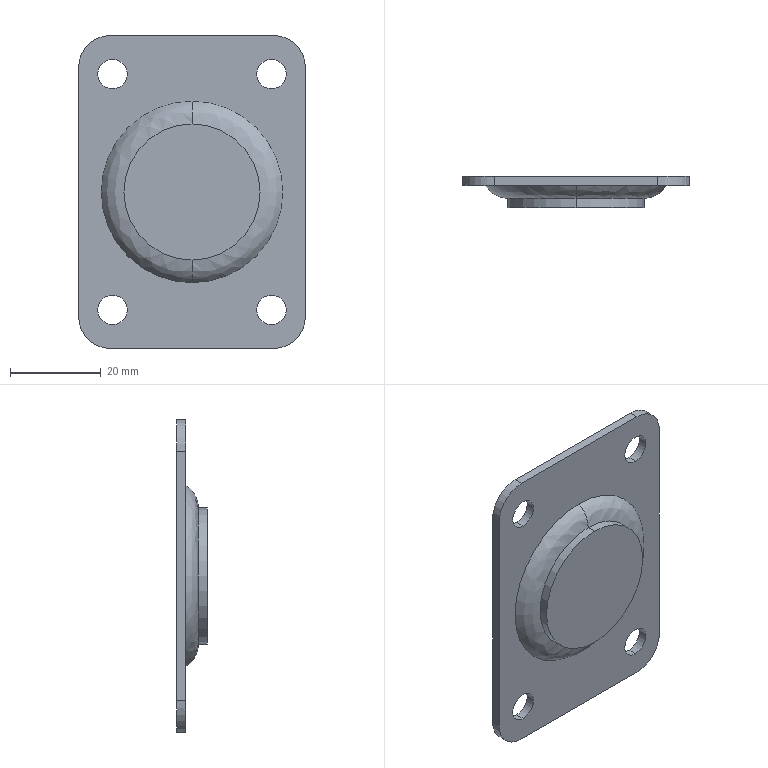Part | STEP file | Caster plate | 1 solid | 46 faces | box 50 x 6.8 x 69 mm | volume 8896 mm3 | cylinder 20 | torus 10 | plane 10 | spline 6 | commonest cylinder face diameters 6.5 x8 14 x4 16 x2 20 x2 30 x2 36 x2
STEP:
#1=CARTESIAN_POINT('',(0.,4.8,20.));
#2=VERTEX_POINT('',#1);
#3=CARTESIAN_POINT('',(0.,4.8,-20.));
#4=VERTEX_POINT('',#3);
#5=CARTESIAN_POINT('',(0.,4.8,0.));
#6=DIRECTION('',(0.,-1.,0.));
#7=DIRECTION('',(0.,0.,1.));
#8=AXIS2_PLACEMENT_3D('',#5,#6,#7);
#9=CIRCLE('',#8,20.);
#10=EDGE_CURVE('',#2,#4,#9,.T.);
#11=ORIENTED_EDGE('',*,*,#10,.T.);
#12=CARTESIAN_POINT('',(0.,2.,-15.));
#13=VERTEX_POINT('',#12);
#14=CARTESIAN_POINT('',(0.,7.864,-15.));
#15=DIRECTION('',(-1.,0.,0.));
#16=DIRECTION('',(0.,0.,-1.));
#17=AXIS2_PLACEMENT_3D('',#14,#15,#16);
#18=CIRCLE('',#17,5.864);
#19=EDGE_CURVE('',#4,#13,#18,.T.);
#20=ORIENTED_EDGE('',*,*,#19,.T.);
#21=CARTESIAN_POINT('',(0.,2.,15.));
#22=VERTEX_POINT('',#21);
#23=CARTESIAN_POINT('',(0.,2.,0.));
#24=DIRECTION('',(0.,1.,0.));
#25=DIRECTION('',(0.,0.,1.));
#26=AXIS2_PLACEMENT_3D('',#23,#24,#25);
#27=CIRCLE('',#26,15.);
#28=EDGE_CURVE('',#13,#22,#27,.T.);
#29=ORIENTED_EDGE('',*,*,#28,.T.);
#30=CARTESIAN_POINT('',(0.,7.864,15.));
#31=DIRECTION('',(1.,0.,0.));
#32=DIRECTION('',(0.,0.,1.));
#33=AXIS2_PLACEMENT_3D('',#30,#31,#32);
#34=CIRCLE('',#33,5.864);
#35=EDGE_CURVE('',#2,#22,#34,.T.);
#36=ORIENTED_EDGE('',*,*,#35,.F.);
#37=EDGE_LOOP('',(#11,#20,#29,#36));
#38=FACE_OUTER_BOUND('',#37,.T.);
#39=CARTESIAN_POINT('',(0.,4.8,-20.));
#40=CARTESIAN_POINT('',(-40.,4.8,-20.));
#41=CARTESIAN_POINT('',(-40.,4.8,20.));
#42=CARTESIAN_POINT('',(0.,4.8,20.));
#43=CARTESIAN_POINT('',(0.,3.02,-18.909));
#44=CARTESIAN_POINT('',(-37.818,3.02,-18.909));
#45=CARTESIAN_POINT('',(-37.818,3.02,18.909));
#46=CARTESIAN_POINT('',(0.,3.02,18.909));
#47=CARTESIAN_POINT('',(0.,2.,-17.088));
#48=CARTESIAN_POINT('',(-34.175,2.,-17.088));
#49=CARTESIAN_POINT('',(-34.175,2.,17.088));
#50=CARTESIAN_POINT('',(0.,2.,17.088));
#51=CARTESIAN_POINT('',(0.,2.,-15.));
#52=CARTESIAN_POINT('',(-30.,2.,-15.));
#53=CARTESIAN_POINT('',(-30.,2.,15.));
#54=CARTESIAN_POINT('',(0.,2.,15.));
#55=(BOUNDED_SURFACE()B_SPLINE_SURFACE(3,3,((#39,#40,#41,#42),(#43,#44,#45,#46),(#47,#48,#49,#50),(#51,#52,#53,#54)),.UNSPECIFIED.,.F.,.F.,.F.)B_SPLINE_SURFACE_WITH_KNOTS((4,4),(4,4),(0.,1.),(0.,1.),.UNSPECIFIED.)GEOMETRIC_REPRESENTATION_ITEM()RATIONAL_B_SPLINE_SURFACE(((1.,0.3333,0.3333,1.),(0.915,0.305,0.305,0.915),(0.915,0.305,0.305,0.915),(1.,0.3333,0.3333,1.)))REPRESENTATION_ITEM('')SURFACE());
#56=ADVANCED_FACE('',(#38),#55,.T.);
#57=CARTESIAN_POINT('',(0.,3.8,15.5));
#58=VERTEX_POINT('',#57);
#59=CARTESIAN_POINT('',(0.,3.8,-15.5));
#60=VERTEX_POINT('',#59);
#61=CARTESIAN_POINT('',(0.,3.8,15.5));
#62=CARTESIAN_POINT('',(31.,3.8,15.5));
#63=CARTESIAN_POINT('',(31.,3.8,-15.5));
#64=CARTESIAN_POINT('',(0.,3.8,-15.5));
#65=(BOUNDED_CURVE()B_SPLINE_CURVE(3,(#61,#62,#63,#64),.UNSPECIFIED.,.F.,.T.)B_SPLINE_CURVE_WITH_KNOTS((4,4),(0.,0.5),.UNSPECIFIED.)CURVE()GEOMETRIC_REPRESENTATION_ITEM()RATIONAL_B_SPLINE_CURVE((1.,0.3333,0.3333,1.))REPRESENTATION_ITEM(''));
#66=EDGE_CURVE('',#58,#60,#65,.T.);
#67=ORIENTED_EDGE('',*,*,#66,.T.);
#68=CARTESIAN_POINT('',(0.,4.3,-15.));
#69=VERTEX_POINT('',#68);
#70=CARTESIAN_POINT('',(0.,4.3,-15.5));
#71=DIRECTION('',(-1.,0.,0.));
#72=DIRECTION('',(0.,0.,-1.));
#73=AXIS2_PLACEMENT_3D('',#70,#71,#72);
#74=CIRCLE('',#73,0.5);
#75=EDGE_CURVE('',#60,#69,#74,.T.);
#76=ORIENTED_EDGE('',*,*,#75,.T.);
#77=CARTESIAN_POINT('',(0.,4.3,15.));
#78=VERTEX_POINT('',#77);
#79=CARTESIAN_POINT('',(0.,4.3,0.));
#80=DIRECTION('',(0.,1.,0.));
#81=DIRECTION('',(0.,0.,1.));
#82=AXIS2_PLACEMENT_3D('',#79,#80,#81);
#83=CIRCLE('',#82,15.);
#84=EDGE_CURVE('',#78,#69,#83,.T.);
#85=ORIENTED_EDGE('',*,*,#84,.F.);
#86=CARTESIAN_POINT('',(0.,4.3,15.5));
#87=DIRECTION('',(1.,0.,0.));
#88=DIRECTION('',(0.,0.,1.));
#89=AXIS2_PLACEMENT_3D('',#86,#87,#88);
#90=CIRCLE('',#89,0.5);
#91=EDGE_CURVE('',#58,#78,#90,.T.);
#92=ORIENTED_EDGE('',*,*,#91,.F.);
#93=EDGE_LOOP('',(#67,#76,#85,#92));
#94=FACE_OUTER_BOUND('',#93,.T.);
#95=CARTESIAN_POINT('',(0.,3.8,15.5));
#96=CARTESIAN_POINT('',(31.,3.8,15.5));
#97=CARTESIAN_POINT('',(31.,3.8,-15.5));
#98=CARTESIAN_POINT('',(0.,3.8,-15.5));
#99=CARTESIAN_POINT('',(0.,3.8,15.207));
#100=CARTESIAN_POINT('',(30.414,3.8,15.207));
#101=CARTESIAN_POINT('',(30.414,3.8,-15.207));
#102=CARTESIAN_POINT('',(0.,3.8,-15.207));
#103=CARTESIAN_POINT('',(0.,4.007,15.));
#104=CARTESIAN_POINT('',(30.,4.007,15.));
#105=CARTESIAN_POINT('',(30.,4.007,-15.));
#106=CARTESIAN_POINT('',(0.,4.007,-15.));
#107=CARTESIAN_POINT('',(0.,4.3,15.));
#108=CARTESIAN_POINT('',(30.,4.3,15.));
#109=CARTESIAN_POINT('',(30.,4.3,-15.));
#110=CARTESIAN_POINT('',(0.,4.3,-15.));
#111=(BOUNDED_SURFACE()B_SPLINE_SURFACE(3,3,((#95,#96,#97,#98),(#99,#100,#101,#102),(#103,#104,#105,#106),(#107,#108,#109,#110)),.UNSPECIFIED.,.F.,.F.,.T.)B_SPLINE_SURFACE_WITH_KNOTS((4,4),(4,4),(0.,1.),(0.,1.),.UNSPECIFIED.)GEOMETRIC_REPRESENTATION_ITEM()RATIONAL_B_SPLINE_SURFACE(((1.,0.3333,0.3333,1.),(0.8047,0.2682,0.2682,0.8047),(0.8047,0.2682,0.2682,0.8047),(1.,0.3333,0.3333,1.)))REPRESENTATION_ITEM('')SURFACE());
#112=ADVANCED_FACE('',(#94),#111,.F.);
#113=CARTESIAN_POINT('',(0.,4.3,10.));
#114=VERTEX_POINT('',#113);
#115=CARTESIAN_POINT('',(0.,4.3,-10.));
#116=VERTEX_POINT('',#115);
#117=CARTESIAN_POINT('',(0.,4.3,0.));
#118=DIRECTION('',(0.,-1.,0.));
#119=DIRECTION('',(0.,0.,1.));
#120=AXIS2_PLACEMENT_3D('',#117,#118,#119);
#121=CIRCLE('',#120,10.);
#122=EDGE_CURVE('',#114,#116,#121,.T.);
#123=ORIENTED_EDGE('',*,*,#122,.T.);
#124=CARTESIAN_POINT('',(0.,2.546,-12.5));
#125=DIRECTION('',(-1.,0.,0.));
#126=DIRECTION('',(0.,0.,-1.));
#127=AXIS2_PLACEMENT_3D('',#124,#125,#126);
#128=CIRCLE('',#127,3.054);
#129=EDGE_CURVE('',#116,#69,#128,.T.);
#130=ORIENTED_EDGE('',*,*,#129,.T.);
#131=CARTESIAN_POINT('',(0.,4.3,0.));
#132=DIRECTION('',(0.,1.,0.));
#133=DIRECTION('',(0.,0.,1.));
#134=AXIS2_PLACEMENT_3D('',#131,#132,#133);
#135=CIRCLE('',#134,15.);
#136=EDGE_CURVE('',#69,#78,#135,.T.);
#137=ORIENTED_EDGE('',*,*,#136,.T.);
#138=CARTESIAN_POINT('',(0.,2.546,12.5));
#139=DIRECTION('',(1.,0.,0.));
#140=DIRECTION('',(0.,0.,1.));
#141=AXIS2_PLACEMENT_3D('',#138,#139,#140);
#142=CIRCLE('',#141,3.054);
#143=EDGE_CURVE('',#114,#78,#142,.T.);
#144=ORIENTED_EDGE('',*,*,#143,.F.);
#145=EDGE_LOOP('',(#123,#130,#137,#144));
#146=FACE_OUTER_BOUND('',#145,.T.);
#147=CARTESIAN_POINT('',(0.,4.3,-10.));
#148=CARTESIAN_POINT('',(-20.,4.3,-10.));
#149=CARTESIAN_POINT('',(-20.,4.3,10.));
#150=CARTESIAN_POINT('',(0.,4.3,10.));
#151=CARTESIAN_POINT('',(0.,6.205,-11.336));
#152=CARTESIAN_POINT('',(-22.673,6.205,-11.336));
#153=CARTESIAN_POINT('',(-22.673,6.205,11.336));
#154=CARTESIAN_POINT('',(0.,6.205,11.336));
#155=CARTESIAN_POINT('',(0.,6.205,-13.664));
#156=CARTESIAN_POINT('',(-27.327,6.205,-13.664));
#157=CARTESIAN_POINT('',(-27.327,6.205,13.664));
#158=CARTESIAN_POINT('',(0.,6.205,13.664));
#159=CARTESIAN_POINT('',(0.,4.3,-15.));
#160=CARTESIAN_POINT('',(-30.,4.3,-15.));
#161=CARTESIAN_POINT('',(-30.,4.3,15.));
#162=CARTESIAN_POINT('',(0.,4.3,15.));
#163=(BOUNDED_SURFACE()B_SPLINE_SURFACE(3,3,((#147,#148,#149,#150),(#151,#152,#153,#154),(#155,#156,#157,#158),(#159,#160,#161,#162)),.UNSPECIFIED.,.F.,.F.,.F.)B_SPLINE_SURFACE_WITH_KNOTS((4,4),(4,4),(0.,1.),(0.,1.),.UNSPECIFIED.)GEOMETRIC_REPRESENTATION_ITEM()RATIONAL_B_SPLINE_SURFACE(((1.,0.3333,0.3333,1.),(0.7162,0.2387,0.2387,0.7162),(0.7162,0.2387,0.2387,0.7162),(1.,0.3333,0.3333,1.)))REPRESENTATION_ITEM('')SURFACE());
#164=ADVANCED_FACE('',(#146),#163,.T.);
#165=CARTESIAN_POINT('',(0.,6.8,-20.));
#166=VERTEX_POINT('',#165);
#167=CARTESIAN_POINT('',(0.,6.8,20.));
#168=VERTEX_POINT('',#167);
#169=CARTESIAN_POINT('',(0.,6.8,0.));
#170=DIRECTION('',(0.,-1.,0.));
#171=DIRECTION('',(0.,0.,1.));
#172=AXIS2_PLACEMENT_3D('',#169,#170,#171);
#173=CIRCLE('',#172,20.);
#174=EDGE_CURVE('',#166,#168,#173,.T.);
#175=ORIENTED_EDGE('',*,*,#174,.F.);
#176=CARTESIAN_POINT('',(0.,4.8,-18.));
#177=VERTEX_POINT('',#176);
#178=CARTESIAN_POINT('',(0.,4.8,-20.));
#179=DIRECTION('',(1.,0.,0.));
#180=DIRECTION('',(0.,0.,-1.));
#181=AXIS2_PLACEMENT_3D('',#178,#179,#180);
#182=CIRCLE('',#181,2.);
#183=EDGE_CURVE('',#166,#177,#182,.T.);
#184=ORIENTED_EDGE('',*,*,#183,.T.);
#185=CARTESIAN_POINT('',(0.,4.8,18.));
#186=VERTEX_POINT('',#185);
#187=CARTESIAN_POINT('',(0.,4.8,0.));
#188=DIRECTION('',(0.,1.,0.));
#189=DIRECTION('',(0.,0.,1.));
#190=AXIS2_PLACEMENT_3D('',#187,#188,#189);
#191=CIRCLE('',#190,18.);
#192=EDGE_CURVE('',#186,#177,#191,.T.);
#193=ORIENTED_EDGE('',*,*,#192,.F.);
#194=CARTESIAN_POINT('',(0.,4.8,20.));
#195=DIRECTION('',(-1.,0.,0.));
#196=DIRECTION('',(0.,0.,1.));
#197=AXIS2_PLACEMENT_3D('',#194,#195,#196);
#198=CIRCLE('',#197,2.);
#199=EDGE_CURVE('',#168,#186,#198,.T.);
#200=ORIENTED_EDGE('',*,*,#199,.F.);
#201=EDGE_LOOP('',(#175,#184,#193,#200));
#202=FACE_OUTER_BOUND('',#201,.T.);
#203=CARTESIAN_POINT('',(0.,4.8,0.));
#204=DIRECTION('',(0.,1.,0.));
#205=DIRECTION('',(0.,0.,1.));
#206=AXIS2_PLACEMENT_3D('',#203,#204,#205);
#207=TOROIDAL_SURFACE('',#206,20.,2.);
#208=ADVANCED_FACE('',(#202),#207,.T.);
#209=CARTESIAN_POINT('',(0.,5.8,-8.));
#210=VERTEX_POINT('',#209);
#211=CARTESIAN_POINT('',(0.,5.8,8.));
#212=VERTEX_POINT('',#211);
#213=CARTESIAN_POINT('',(0.,5.8,0.));
#214=DIRECTION('',(0.,-1.,0.));
#215=DIRECTION('',(0.,0.,1.));
#216=AXIS2_PLACEMENT_3D('',#213,#214,#215);
#217=CIRCLE('',#216,8.);
#218=EDGE_CURVE('',#210,#212,#217,.T.);
#219=ORIENTED_EDGE('',*,*,#218,.F.);
#220=CARTESIAN_POINT('',(0.,6.8,-7.));
#221=VERTEX_POINT('',#220);
#222=CARTESIAN_POINT('',(0.,5.8,-7.));
#223=DIRECTION('',(1.,0.,0.));
#224=DIRECTION('',(0.,0.,-1.));
#225=AXIS2_PLACEMENT_3D('',#222,#223,#224);
#226=CIRCLE('',#225,1.);
#227=EDGE_CURVE('',#210,#221,#226,.T.);
#228=ORIENTED_EDGE('',*,*,#227,.T.);
#229=CARTESIAN_POINT('',(0.,6.8,7.));
#230=VERTEX_POINT('',#229);
#231=CARTESIAN_POINT('',(0.,6.8,0.));
#232=DIRECTION('',(0.,1.,0.));
#233=DIRECTION('',(0.,0.,1.));
#234=AXIS2_PLACEMENT_3D('',#231,#232,#233);
#235=CIRCLE('',#234,7.);
#236=EDGE_CURVE('',#230,#221,#235,.T.);
#237=ORIENTED_EDGE('',*,*,#236,.F.);
#238=CARTESIAN_POINT('',(0.,5.8,7.));
#239=DIRECTION('',(-1.,0.,0.));
#240=DIRECTION('',(0.,0.,1.));
#241=AXIS2_PLACEMENT_3D('',#238,#239,#240);
#242=CIRCLE('',#241,1.);
#243=EDGE_CURVE('',#212,#230,#242,.T.);
#244=ORIENTED_EDGE('',*,*,#243,.F.);
#245=EDGE_LOOP('',(#219,#228,#237,#244));
#246=FACE_OUTER_BOUND('',#245,.T.);
#247=CARTESIAN_POINT('',(0.,5.8,0.));
#248=DIRECTION('',(0.,1.,0.));
#249=DIRECTION('',(0.,0.,1.));
#250=AXIS2_PLACEMENT_3D('',#247,#248,#249);
#251=TOROIDAL_SURFACE('',#250,7.,1.);
#252=ADVANCED_FACE('',(#246),#251,.T.);
#253=CARTESIAN_POINT('',(0.,4.3,18.));
#254=VERTEX_POINT('',#253);
#255=CARTESIAN_POINT('',(0.,4.3,-18.));
#256=VERTEX_POINT('',#255);
#257=CARTESIAN_POINT('',(0.,4.3,0.));
#258=DIRECTION('',(0.,-1.,0.));
#259=DIRECTION('',(0.,0.,-1.));
#260=AXIS2_PLACEMENT_3D('',#257,#258,#259);
#261=CIRCLE('',#260,18.);
#262=EDGE_CURVE('',#254,#256,#261,.T.);
#263=ORIENTED_EDGE('',*,*,#262,.F.);
#264=CARTESIAN_POINT('',(0.,3.8,17.5));
#265=VERTEX_POINT('',#264);
#266=CARTESIAN_POINT('',(0.,4.3,17.5));
#267=DIRECTION('',(1.,0.,0.));
#268=DIRECTION('',(0.,0.,-1.));
#269=AXIS2_PLACEMENT_3D('',#266,#267,#268);
#270=CIRCLE('',#269,0.5);
#271=EDGE_CURVE('',#254,#265,#270,.T.);
#272=ORIENTED_EDGE('',*,*,#271,.T.);
#273=CARTESIAN_POINT('',(0.,3.8,-17.5));
#274=VERTEX_POINT('',#273);
#275=CARTESIAN_POINT('',(0.,3.8,0.));
#276=DIRECTION('',(0.,1.,0.));
#277=DIRECTION('',(0.,0.,-1.));
#278=AXIS2_PLACEMENT_3D('',#275,#276,#277);
#279=CIRCLE('',#278,17.5);
#280=EDGE_CURVE('',#274,#265,#279,.T.);
#281=ORIENTED_EDGE('',*,*,#280,.F.);
#282=CARTESIAN_POINT('',(0.,4.3,-17.5));
#283=DIRECTION('',(-1.,0.,0.));
#284=DIRECTION('',(0.,0.,1.));
#285=AXIS2_PLACEMENT_3D('',#282,#283,#284);
#286=CIRCLE('',#285,0.5);
#287=EDGE_CURVE('',#256,#274,#286,.T.);
#288=ORIENTED_EDGE('',*,*,#287,.F.);
#289=EDGE_LOOP('',(#263,#272,#281,#288));
#290=FACE_OUTER_BOUND('',#289,.T.);
#291=CARTESIAN_POINT('',(0.,4.3,0.));
#292=DIRECTION('',(0.,-1.,0.));
#293=DIRECTION('',(0.,0.,-1.));
#294=AXIS2_PLACEMENT_3D('',#291,#292,#293);
#295=TOROIDAL_SURFACE('',#294,17.5,0.5);
#296=ADVANCED_FACE('',(#290),#295,.F.);
#297=CARTESIAN_POINT('',(0.,2.8,8.5));
#298=VERTEX_POINT('',#297);
#299=CARTESIAN_POINT('',(0.,2.8,-8.5));
#300=VERTEX_POINT('',#299);
#301=CARTESIAN_POINT('',(0.,2.8,0.));
#302=DIRECTION('',(0.,-1.,0.));
#303=DIRECTION('',(0.,0.,-1.));
#304=AXIS2_PLACEMENT_3D('',#301,#302,#303);
#305=CIRCLE('',#304,8.5);
#306=EDGE_CURVE('',#298,#300,#305,.T.);
#307=ORIENTED_EDGE('',*,*,#306,.F.);
#308=CARTESIAN_POINT('',(0.,3.3,8.));
#309=VERTEX_POINT('',#308);
#310=CARTESIAN_POINT('',(0.,3.3,8.5));
#311=DIRECTION('',(1.,0.,0.));
#312=DIRECTION('',(0.,0.,-1.));
#313=AXIS2_PLACEMENT_3D('',#310,#311,#312);
#314=CIRCLE('',#313,0.5);
#315=EDGE_CURVE('',#298,#309,#314,.T.);
#316=ORIENTED_EDGE('',*,*,#315,.T.);
#317=CARTESIAN_POINT('',(0.,3.3,-8.));
#318=VERTEX_POINT('',#317);
#319=CARTESIAN_POINT('',(0.,3.3,0.));
#320=DIRECTION('',(0.,1.,0.));
#321=DIRECTION('',(0.,0.,-1.));
#322=AXIS2_PLACEMENT_3D('',#319,#320,#321);
#323=CIRCLE('',#322,8.);
#324=EDGE_CURVE('',#318,#309,#323,.T.);
#325=ORIENTED_EDGE('',*,*,#324,.F.);
#326=CARTESIAN_POINT('',(0.,3.3,-8.5));
#327=DIRECTION('',(-1.,0.,0.));
#328=DIRECTION('',(0.,0.,1.));
#329=AXIS2_PLACEMENT_3D('',#326,#327,#328);
#330=CIRCLE('',#329,0.5);
#331=EDGE_CURVE('',#300,#318,#330,.T.);
#332=ORIENTED_EDGE('',*,*,#331,.F.);
#333=EDGE_LOOP('',(#307,#316,#325,#332));
#334=FACE_OUTER_BOUND('',#333,.T.);
#335=CARTESIAN_POINT('',(0.,3.3,0.));
#336=DIRECTION('',(0.,-1.,0.));
#337=DIRECTION('',(0.,0.,-1.));
#338=AXIS2_PLACEMENT_3D('',#335,#336,#337);
#339=TOROIDAL_SURFACE('',#338,8.5,0.5);
#340=ADVANCED_FACE('',(#334),#339,.F.);
#341=CARTESIAN_POINT('',(0.,3.3,10.));
#342=VERTEX_POINT('',#341);
#343=CARTESIAN_POINT('',(0.,3.3,-10.));
#344=VERTEX_POINT('',#343);
#345=CARTESIAN_POINT('',(0.,3.3,0.));
#346=DIRECTION('',(0.,-1.,0.));
#347=DIRECTION('',(0.,0.,-1.));
#348=AXIS2_PLACEMENT_3D('',#345,#346,#347);
#349=CIRCLE('',#348,10.);
#350=EDGE_CURVE('',#342,#344,#349,.T.);
#351=ORIENTED_EDGE('',*,*,#350,.F.);
#352=CARTESIAN_POINT('',(0.,2.8,9.5));
#353=VERTEX_POINT('',#352);
#354=CARTESIAN_POINT('',(0.,3.3,9.5));
#355=DIRECTION('',(1.,0.,0.));
#356=DIRECTION('',(0.,0.,-1.));
#357=AXIS2_PLACEMENT_3D('',#354,#355,#356);
#358=CIRCLE('',#357,0.5);
#359=EDGE_CURVE('',#342,#353,#358,.T.);
#360=ORIENTED_EDGE('',*,*,#359,.T.);
#361=CARTESIAN_POINT('',(0.,2.8,-9.5));
#362=VERTEX_POINT('',#361);
#363=CARTESIAN_POINT('',(0.,2.8,0.));
#364=DIRECTION('',(0.,1.,0.));
#365=DIRECTION('',(0.,0.,-1.));
#366=AXIS2_PLACEMENT_3D('',#363,#364,#365);
#367=CIRCLE('',#366,9.5);
#368=EDGE_CURVE('',#362,#353,#367,.T.);
#369=ORIENTED_EDGE('',*,*,#368,.F.);
#370=CARTESIAN_POINT('',(0.,3.3,-9.5));
#371=DIRECTION('',(-1.,0.,0.));
#372=DIRECTION('',(0.,0.,1.));
#373=AXIS2_PLACEMENT_3D('',#370,#371,#372);
#374=CIRCLE('',#373,0.5);
#375=EDGE_CURVE('',#344,#362,#374,.T.);
#376=ORIENTED_EDGE('',*,*,#375,.F.);
#377=EDGE_LOOP('',(#351,#360,#369,#376));
#378=FACE_OUTER_BOUND('',#377,.T.);
#379=CARTESIAN_POINT('',(0.,3.3,0.));
#380=DIRECTION('',(0.,-1.,0.));
#381=DIRECTION('',(0.,0.,-1.));
#382=AXIS2_PLACEMENT_3D('',#379,#380,#381);
#383=TOROIDAL_SURFACE('',#382,9.5,0.5);
#384=ADVANCED_FACE('',(#378),#383,.F.);
#385=CARTESIAN_POINT('',(17.5,6.8,-22.75));
#386=VERTEX_POINT('',#385);
#387=CARTESIAN_POINT('',(17.5,6.8,-29.25));
#388=VERTEX_POINT('',#387);
#389=CARTESIAN_POINT('',(17.5,6.8,-26.));
#390=DIRECTION('',(0.,-1.,0.));
#391=DIRECTION('',(0.,0.,-1.));
#392=AXIS2_PLACEMENT_3D('',#389,#390,#391);
#393=CIRCLE('',#392,3.25);
#394=EDGE_CURVE('',#386,#388,#393,.T.);
#395=ORIENTED_EDGE('',*,*,#394,.F.);
#396=CARTESIAN_POINT('',(17.5,4.8,-22.75));
#397=VERTEX_POINT('',#396);
#398=CARTESIAN_POINT('',(17.5,4.8,-22.75));
#399=DIRECTION('',(0.,-1.,0.));
#400=VECTOR('',#399,1000.);
#401=LINE('',#398,#400);
#402=EDGE_CURVE('',#386,#397,#401,.T.);
#403=ORIENTED_EDGE('',*,*,#402,.T.);
#404=CARTESIAN_POINT('',(17.5,4.8,-29.25));
#405=VERTEX_POINT('',#404);
#406=CARTESIAN_POINT('',(17.5,4.8,-26.));
#407=DIRECTION('',(0.,-1.,0.));
#408=DIRECTION('',(0.,0.,-1.));
#409=AXIS2_PLACEMENT_3D('',#406,#407,#408);
#410=CIRCLE('',#409,3.25);
#411=EDGE_CURVE('',#397,#405,#410,.T.);
#412=ORIENTED_EDGE('',*,*,#411,.T.);
#413=CARTESIAN_POINT('',(17.5,4.8,-29.25));
#414=DIRECTION('',(0.,-1.,0.));
#415=VECTOR('',#414,1000.);
#416=LINE('',#413,#415);
#417=EDGE_CURVE('',#388,#405,#416,.T.);
#418=ORIENTED_EDGE('',*,*,#417,.F.);
#419=EDGE_LOOP('',(#395,#403,#412,#418));
#420=FACE_OUTER_BOUND('',#419,.T.);
#421=CARTESIAN_POINT('',(17.5,4.8,-26.));
#422=DIRECTION('',(0.,-1.,0.));
#423=DIRECTION('',(0.,0.,-1.));
#424=AXIS2_PLACEMENT_3D('',#421,#422,#423);
#425=CYLINDRICAL_SURFACE('',#424,3.25);
#426=ADVANCED_FACE('',(#420),#425,.F.);
#427=CARTESIAN_POINT('',(-17.5,6.8,29.25));
#428=VERTEX_POINT('',#427);
#429=CARTESIAN_POINT('',(-17.5,6.8,22.75));
#430=VERTEX_POINT('',#429);
#431=CARTESIAN_POINT('',(-17.5,6.8,26.));
#432=DIRECTION('',(0.,-1.,0.));
#433=DIRECTION('',(0.,0.,-1.));
#434=AXIS2_PLACEMENT_3D('',#431,#432,#433);
#435=CIRCLE('',#434,3.25);
#436=EDGE_CURVE('',#428,#430,#435,.T.);
#437=ORIENTED_EDGE('',*,*,#436,.F.);
#438=CARTESIAN_POINT('',(-17.5,4.8,29.25));
#439=VERTEX_POINT('',#438);
#440=CARTESIAN_POINT('',(-17.5,4.8,29.25));
#441=DIRECTION('',(0.,-1.,0.));
#442=VECTOR('',#441,1000.);
#443=LINE('',#440,#442);
#444=EDGE_CURVE('',#428,#439,#443,.T.);
#445=ORIENTED_EDGE('',*,*,#444,.T.);
#446=CARTESIAN_POINT('',(-17.5,4.8,22.75));
#447=VERTEX_POINT('',#446);
#448=CARTESIAN_POINT('',(-17.5,4.8,26.));
#449=DIRECTION('',(0.,-1.,0.));
#450=DIRECTION('',(0.,0.,-1.));
#451=AXIS2_PLACEMENT_3D('',#448,#449,#450);
#452=CIRCLE('',#451,3.25);
#453=EDGE_CURVE('',#439,#447,#452,.T.);
#454=ORIENTED_EDGE('',*,*,#453,.T.);
#455=CARTESIAN_POINT('',(-17.5,4.8,22.75));
#456=DIRECTION('',(0.,-1.,0.));
#457=VECTOR('',#456,1000.);
#458=LINE('',#455,#457);
#459=EDGE_CURVE('',#430,#447,#458,.T.);
#460=ORIENTED_EDGE('',*,*,#459,.F.);
#461=EDGE_LOOP('',(#437,#445,#454,#460));
#462=FACE_OUTER_BOUND('',#461,.T.);
#463=CARTESIAN_POINT('',(-17.5,4.8,26.));
#464=DIRECTION('',(0.,-1.,0.));
#465=DIRECTION('',(0.,0.,-1.));
#466=AXIS2_PLACEMENT_3D('',#463,#464,#465);
#467=CYLINDRICAL_SURFACE('',#466,3.25);
#468=ADVANCED_FACE('',(#462),#467,.F.);
#469=CARTESIAN_POINT('',(-17.5,6.8,-22.75));
#470=VERTEX_POINT('',#469);
#471=CARTESIAN_POINT('',(-17.5,6.8,-29.25));
#472=VERTEX_POINT('',#471);
#473=CARTESIAN_POINT('',(-17.5,6.8,-26.));
#474=DIRECTION('',(0.,-1.,0.));
#475=DIRECTION('',(0.,0.,-1.));
#476=AXIS2_PLACEMENT_3D('',#473,#474,#475);
#477=CIRCLE('',#476,3.25);
#478=EDGE_CURVE('',#470,#472,#477,.T.);
#479=ORIENTED_EDGE('',*,*,#478,.F.);
#480=CARTESIAN_POINT('',(-17.5,4.8,-22.75));
#481=VERTEX_POINT('',#480);
#482=CARTESIAN_POINT('',(-17.5,4.8,-22.75));
#483=DIRECTION('',(0.,-1.,0.));
#484=VECTOR('',#483,1000.);
#485=LINE('',#482,#484);
#486=EDGE_CURVE('',#470,#481,#485,.T.);
#487=ORIENTED_EDGE('',*,*,#486,.T.);
#488=CARTESIAN_POINT('',(-17.5,4.8,-29.25));
#489=VERTEX_POINT('',#488);
#490=CARTESIAN_POINT('',(-17.5,4.8,-26.));
#491=DIRECTION('',(0.,-1.,0.));
#492=DIRECTION('',(0.,0.,-1.));
#493=AXIS2_PLACEMENT_3D('',#490,#491,#492);
#494=CIRCLE('',#493,3.25);
#495=EDGE_CURVE('',#481,#489,#494,.T.);
#496=ORIENTED_EDGE('',*,*,#495,.T.);
#497=CARTESIAN_POINT('',(-17.5,4.8,-29.25));
#498=DIRECTION('',(0.,-1.,0.));
#499=VECTOR('',#498,1000.);
#500=LINE('',#497,#499);
#501=EDGE_CURVE('',#472,#489,#500,.T.);
#502=ORIENTED_EDGE('',*,*,#501,.F.);
#503=EDGE_LOOP('',(#479,#487,#496,#502));
#504=FACE_OUTER_BOUND('',#503,.T.);
#505=CARTESIAN_POINT('',(-17.5,4.8,-26.));
#506=DIRECTION('',(0.,-1.,0.));
#507=DIRECTION('',(0.,0.,-1.));
#508=AXIS2_PLACEMENT_3D('',#505,#506,#507);
#509=CYLINDRICAL_SURFACE('',#508,3.25);
#510=ADVANCED_FACE('',(#504),#509,.F.);
#511=CARTESIAN_POINT('',(17.5,6.8,29.25));
#512=VERTEX_POINT('',#511);
#513=CARTESIAN_POINT('',(17.5,6.8,22.75));
#514=VERTEX_POINT('',#513);
#515=CARTESIAN_POINT('',(17.5,6.8,26.));
#516=DIRECTION('',(0.,-1.,0.));
#517=DIRECTION('',(0.,0.,-1.));
#518=AXIS2_PLACEMENT_3D('',#515,#516,#517);
#519=CIRCLE('',#518,3.25);
#520=EDGE_CURVE('',#512,#514,#519,.T.);
#521=ORIENTED_EDGE('',*,*,#520,.F.);
#522=CARTESIAN_POINT('',(17.5,4.8,29.25));
#523=VERTEX_POINT('',#522);
#524=CARTESIAN_POINT('',(17.5,4.8,29.25));
#525=DIRECTION('',(0.,-1.,0.));
#526=VECTOR('',#525,1000.);
#527=LINE('',#524,#526);
#528=EDGE_CURVE('',#512,#523,#527,.T.);
#529=ORIENTED_EDGE('',*,*,#528,.T.);
#530=CARTESIAN_POINT('',(17.5,4.8,22.75));
#531=VERTEX_POINT('',#530);
#532=CARTESIAN_POINT('',(17.5,4.8,26.));
#533=DIRECTION('',(0.,-1.,0.));
#534=DIRECTION('',(0.,0.,-1.));
#535=AXIS2_PLACEMENT_3D('',#532,#533,#534);
#536=CIRCLE('',#535,3.25);
#537=EDGE_CURVE('',#523,#531,#536,.T.);
#538=ORIENTED_EDGE('',*,*,#537,.T.);
#539=CARTESIAN_POINT('',(17.5,4.8,22.75));
#540=DIRECTION('',(0.,-1.,0.));
#541=VECTOR('',#540,1000.);
#542=LINE('',#539,#541);
#543=EDGE_CURVE('',#514,#531,#542,.T.);
#544=ORIENTED_EDGE('',*,*,#543,.F.);
#545=EDGE_LOOP('',(#521,#529,#538,#544));
#546=FACE_OUTER_BOUND('',#545,.T.);
#547=CARTESIAN_POINT('',(17.5,4.8,26.));
#548=DIRECTION('',(0.,-1.,0.));
#549=DIRECTION('',(0.,0.,-1.));
#550=AXIS2_PLACEMENT_3D('',#547,#548,#549);
#551=CYLINDRICAL_SURFACE('',#550,3.25);
#552=ADVANCED_FACE('',(#546),#551,.F.);
#553=ORIENTED_EDGE('',*,*,#218,.T.);
#554=CARTESIAN_POINT('',(0.,6.8,8.));
#555=DIRECTION('',(0.,-1.,0.));
#556=VECTOR('',#555,1000.);
#557=LINE('',#554,#556);
#558=EDGE_CURVE('',#212,#309,#557,.T.);
#559=ORIENTED_EDGE('',*,*,#558,.T.);
#560=CARTESIAN_POINT('',(0.,3.3,0.));
#561=DIRECTION('',(0.,1.,0.));
#562=DIRECTION('',(0.,0.,-1.));
#563=AXIS2_PLACEMENT_3D('',#560,#561,#562);
#564=CIRCLE('',#563,8.);
#565=EDGE_CURVE('',#309,#318,#564,.T.);
#566=ORIENTED_EDGE('',*,*,#565,.T.);
#567=CARTESIAN_POINT('',(0.,6.8,-8.));
#568=DIRECTION('',(0.,-1.,0.));
#569=VECTOR('',#568,1000.);
#570=LINE('',#567,#569);
#571=EDGE_CURVE('',#210,#318,#570,.T.);
#572=ORIENTED_EDGE('',*,*,#571,.F.);
#573=EDGE_LOOP('',(#553,#559,#566,#572));
#574=FACE_OUTER_BOUND('',#573,.T.);
#575=CARTESIAN_POINT('',(0.,6.8,0.));
#576=DIRECTION('',(0.,-1.,0.));
#577=DIRECTION('',(0.,0.,-1.));
#578=AXIS2_PLACEMENT_3D('',#575,#576,#577);
#579=CYLINDRICAL_SURFACE('',#578,8.);
#580=ADVANCED_FACE('',(#574),#579,.T.);
#581=CARTESIAN_POINT('',(0.,4.8,0.));
#582=DIRECTION('',(0.,1.,0.));
#583=DIRECTION('',(0.,0.,1.));
#584=AXIS2_PLACEMENT_3D('',#581,#582,#583);
#585=CIRCLE('',#584,18.);
#586=EDGE_CURVE('',#177,#186,#585,.T.);
#587=ORIENTED_EDGE('',*,*,#586,.T.);
#588=CARTESIAN_POINT('',(0.,50.,18.));
#589=DIRECTION('',(0.,-1.,0.));
#590=VECTOR('',#589,1000.);
#591=LINE('',#588,#590);
#592=EDGE_CURVE('',#186,#254,#591,.T.);
#593=ORIENTED_EDGE('',*,*,#592,.T.);
#594=ORIENTED_EDGE('',*,*,#262,.T.);
#595=CARTESIAN_POINT('',(0.,50.,-18.));
#596=DIRECTION('',(0.,-1.,0.));
#597=VECTOR('',#596,1000.);
#598=LINE('',#595,#597);
#599=EDGE_CURVE('',#177,#256,#598,.T.);
#600=ORIENTED_EDGE('',*,*,#599,.F.);
#601=EDGE_LOOP('',(#587,#593,#594,#600));
#602=FACE_OUTER_BOUND('',#601,.T.);
#603=CARTESIAN_POINT('',(0.,50.,0.));
#604=DIRECTION('',(0.,-1.,0.));
#605=DIRECTION('',(0.,0.,-1.));
#606=AXIS2_PLACEMENT_3D('',#603,#604,#605);
#607=CYLINDRICAL_SURFACE('',#606,18.);
#608=ADVANCED_FACE('',(#602),#607,.F.);
#609=CARTESIAN_POINT('',(0.,2.,0.));
#610=DIRECTION('',(0.,1.,0.));
#611=DIRECTION('',(0.,0.,1.));
#612=AXIS2_PLACEMENT_3D('',#609,#610,#611);
#613=CIRCLE('',#612,15.);
#614=EDGE_CURVE('',#22,#13,#613,.T.);
#615=ORIENTED_EDGE('',*,*,#614,.F.);
#616=CARTESIAN_POINT('',(0.,0.,15.));
#617=VERTEX_POINT('',#616);
#618=CARTESIAN_POINT('',(0.,4.8,15.));
#619=DIRECTION('',(0.,-1.,0.));
#620=VECTOR('',#619,1000.);
#621=LINE('',#618,#620);
#622=EDGE_CURVE('',#22,#617,#621,.T.);
#623=ORIENTED_EDGE('',*,*,#622,.T.);
#624=CARTESIAN_POINT('',(0.,0.,-15.));
#625=VERTEX_POINT('',#624);
#626=CARTESIAN_POINT('',(0.,0.,0.));
#627=DIRECTION('',(0.,1.,0.));
#628=DIRECTION('',(0.,0.,-1.));
#629=AXIS2_PLACEMENT_3D('',#626,#627,#628);
#630=CIRCLE('',#629,15.);
#631=EDGE_CURVE('',#617,#625,#630,.T.);
#632=ORIENTED_EDGE('',*,*,#631,.T.);
#633=CARTESIAN_POINT('',(0.,4.8,-15.));
#634=DIRECTION('',(0.,-1.,0.));
#635=VECTOR('',#634,1000.);
#636=LINE('',#633,#635);
#637=EDGE_CURVE('',#13,#625,#636,.T.);
#638=ORIENTED_EDGE('',*,*,#637,.F.);
#639=EDGE_LOOP('',(#615,#623,#632,#638));
#640=FACE_OUTER_BOUND('',#639,.T.);
#641=CARTESIAN_POINT('',(0.,4.8,0.));
#642=DIRECTION('',(0.,-1.,0.));
#643=DIRECTION('',(0.,0.,-1.));
#644=AXIS2_PLACEMENT_3D('',#641,#642,#643);
#645=CYLINDRICAL_SURFACE('',#644,15.);
#646=ADVANCED_FACE('',(#640),#645,.T.);
#647=ORIENTED_EDGE('',*,*,#122,.F.);
#648=CARTESIAN_POINT('',(0.,50.,10.));
#649=DIRECTION('',(0.,-1.,0.));
#650=VECTOR('',#649,1000.);
#651=LINE('',#648,#650);
#652=EDGE_CURVE('',#114,#342,#651,.T.);
#653=ORIENTED_EDGE('',*,*,#652,.T.);
#654=ORIENTED_EDGE('',*,*,#350,.T.);
#655=CARTESIAN_POINT('',(0.,50.,-10.));
#656=DIRECTION('',(0.,-1.,0.));
#657=VECTOR('',#656,1000.);
#658=LINE('',#655,#657);
#659=EDGE_CURVE('',#116,#344,#658,.T.);
#660=ORIENTED_EDGE('',*,*,#659,.F.);
#661=EDGE_LOOP('',(#647,#653,#654,#660));
#662=FACE_OUTER_BOUND('',#661,.T.);
#663=CARTESIAN_POINT('',(0.,50.,0.));
#664=DIRECTION('',(0.,-1.,0.));
#665=DIRECTION('',(0.,0.,-1.));
#666=AXIS2_PLACEMENT_3D('',#663,#664,#665);
#667=CYLINDRICAL_SURFACE('',#666,10.);
#668=ADVANCED_FACE('',(#662),#667,.F.);
#669=CARTESIAN_POINT('',(0.,6.8,0.));
#670=DIRECTION('',(0.,-1.,0.));
#671=DIRECTION('',(0.,0.,1.));
#672=AXIS2_PLACEMENT_3D('',#669,#670,#671);
#673=CIRCLE('',#672,20.);
#674=EDGE_CURVE('',#168,#166,#673,.T.);
#675=ORIENTED_EDGE('',*,*,#674,.T.);
#676=ORIENTED_EDGE('',*,*,#174,.T.);
#677=EDGE_LOOP('',(#675,#676));
#678=FACE_BOUND('',#677,.T.);
#679=CARTESIAN_POINT('',(17.5,6.8,-26.));
#680=DIRECTION('',(0.,-1.,0.));
#681=DIRECTION('',(0.,0.,-1.));
#682=AXIS2_PLACEMENT_3D('',#679,#680,#681);
#683=CIRCLE('',#682,3.25);
#684=EDGE_CURVE('',#388,#386,#683,.T.);
#685=ORIENTED_EDGE('',*,*,#684,.T.);
#686=ORIENTED_EDGE('',*,*,#394,.T.);
#687=EDGE_LOOP('',(#685,#686));
#688=FACE_BOUND('',#687,.T.);
#689=CARTESIAN_POINT('',(-17.5,6.8,26.));
#690=DIRECTION('',(0.,-1.,0.));
#691=DIRECTION('',(0.,0.,-1.));
#692=AXIS2_PLACEMENT_3D('',#689,#690,#691);
#693=CIRCLE('',#692,3.25);
#694=EDGE_CURVE('',#430,#428,#693,.T.);
#695=ORIENTED_EDGE('',*,*,#694,.T.);
#696=ORIENTED_EDGE('',*,*,#436,.T.);
#697=EDGE_LOOP('',(#695,#696));
#698=FACE_BOUND('',#697,.T.);
#699=CARTESIAN_POINT('',(-17.5,6.8,-26.));
#700=DIRECTION('',(0.,-1.,0.));
#701=DIRECTION('',(0.,0.,-1.));
#702=AXIS2_PLACEMENT_3D('',#699,#700,#701);
#703=CIRCLE('',#702,3.25);
#704=EDGE_CURVE('',#472,#470,#703,.T.);
#705=ORIENTED_EDGE('',*,*,#704,.T.);
#706=ORIENTED_EDGE('',*,*,#478,.T.);
#707=EDGE_LOOP('',(#705,#706));
#708=FACE_BOUND('',#707,.T.);
#709=CARTESIAN_POINT('',(17.5,6.8,26.));
#710=DIRECTION('',(0.,-1.,0.));
#711=DIRECTION('',(0.,0.,-1.));
#712=AXIS2_PLACEMENT_3D('',#709,#710,#711);
#713=CIRCLE('',#712,3.25);
#714=EDGE_CURVE('',#514,#512,#713,.T.);
#715=ORIENTED_EDGE('',*,*,#714,.T.);
#716=ORIENTED_EDGE('',*,*,#520,.T.);
#717=EDGE_LOOP('',(#715,#716));
#718=FACE_BOUND('',#717,.T.);
#719=CARTESIAN_POINT('',(-18.,6.8,-34.5));
#720=VERTEX_POINT('',#719);
#721=CARTESIAN_POINT('',(18.,6.8,-34.5));
#722=VERTEX_POINT('',#721);
#723=CARTESIAN_POINT('',(-32.,6.8,-34.5));
#724=DIRECTION('',(1.,0.,0.));
#725=VECTOR('',#724,1000.);
#726=LINE('',#723,#725);
#727=EDGE_CURVE('',#720,#722,#726,.T.);
#728=ORIENTED_EDGE('',*,*,#727,.F.);
#729=CARTESIAN_POINT('',(-25.,6.8,-27.5));
#730=VERTEX_POINT('',#729);
#731=CARTESIAN_POINT('',(-18.,6.8,-27.5));
#732=DIRECTION('',(0.,1.,0.));
#733=DIRECTION('',(0.,0.,1.));
#734=AXIS2_PLACEMENT_3D('',#731,#732,#733);
#735=CIRCLE('',#734,7.);
#736=EDGE_CURVE('',#720,#730,#735,.T.);
#737=ORIENTED_EDGE('',*,*,#736,.T.);
#738=CARTESIAN_POINT('',(-25.,6.8,27.5));
#739=VERTEX_POINT('',#738);
#740=CARTESIAN_POINT('',(-25.,6.8,-32.));
#741=DIRECTION('',(0.,0.,-1.));
#742=VECTOR('',#741,1000.);
#743=LINE('',#740,#742);
#744=EDGE_CURVE('',#739,#730,#743,.T.);
#745=ORIENTED_EDGE('',*,*,#744,.F.);
#746=CARTESIAN_POINT('',(-18.,6.8,34.5));
#747=VERTEX_POINT('',#746);
#748=CARTESIAN_POINT('',(-18.,6.8,27.5));
#749=DIRECTION('',(0.,1.,0.));
#750=DIRECTION('',(0.,0.,1.));
#751=AXIS2_PLACEMENT_3D('',#748,#749,#750);
#752=CIRCLE('',#751,7.);
#753=EDGE_CURVE('',#739,#747,#752,.T.);
#754=ORIENTED_EDGE('',*,*,#753,.T.);
#755=CARTESIAN_POINT('',(18.,6.8,34.5));
#756=VERTEX_POINT('',#755);
#757=CARTESIAN_POINT('',(-32.,6.8,34.5));
#758=DIRECTION('',(-1.,0.,0.));
#759=VECTOR('',#758,1000.);
#760=LINE('',#757,#759);
#761=EDGE_CURVE('',#756,#747,#760,.T.);
#762=ORIENTED_EDGE('',*,*,#761,.F.);
#763=CARTESIAN_POINT('',(25.,6.8,27.5));
#764=VERTEX_POINT('',#763);
#765=CARTESIAN_POINT('',(18.,6.8,27.5));
#766=DIRECTION('',(0.,1.,0.));
#767=DIRECTION('',(0.,0.,1.));
#768=AXIS2_PLACEMENT_3D('',#765,#766,#767);
#769=CIRCLE('',#768,7.);
#770=EDGE_CURVE('',#756,#764,#769,.T.);
#771=ORIENTED_EDGE('',*,*,#770,.T.);
#772=CARTESIAN_POINT('',(25.,6.8,-27.5));
#773=VERTEX_POINT('',#772);
#774=CARTESIAN_POINT('',(25.,6.8,-32.));
#775=DIRECTION('',(0.,0.,1.));
#776=VECTOR('',#775,1000.);
#777=LINE('',#774,#776);
#778=EDGE_CURVE('',#773,#764,#777,.T.);
#779=ORIENTED_EDGE('',*,*,#778,.F.);
#780=CARTESIAN_POINT('',(18.,6.8,-27.5));
#781=DIRECTION('',(0.,1.,0.));
#782=DIRECTION('',(0.,0.,1.));
#783=AXIS2_PLACEMENT_3D('',#780,#781,#782);
#784=CIRCLE('',#783,7.);
#785=EDGE_CURVE('',#773,#722,#784,.T.);
#786=ORIENTED_EDGE('',*,*,#785,.T.);
#787=EDGE_LOOP('',(#728,#737,#745,#754,#762,#771,#779,#786));
#788=FACE_OUTER_BOUND('',#787,.T.);
#789=CARTESIAN_POINT('',(-32.,6.8,-32.));
#790=DIRECTION('',(0.,1.,0.));
#791=DIRECTION('',(0.,0.,1.));
#792=AXIS2_PLACEMENT_3D('',#789,#790,#791);
#793=PLANE('',#792);
#794=ADVANCED_FACE('',(#678,#688,#698,#708,#718,#788),#793,.T.);
#795=CARTESIAN_POINT('',(17.5,4.8,-26.));
#796=DIRECTION('',(0.,-1.,0.));
#797=DIRECTION('',(0.,0.,-1.));
#798=AXIS2_PLACEMENT_3D('',#795,#796,#797);
#799=CIRCLE('',#798,3.25);
#800=EDGE_CURVE('',#405,#397,#799,.T.);
#801=ORIENTED_EDGE('',*,*,#800,.F.);
#802=ORIENTED_EDGE('',*,*,#411,.F.);
#803=EDGE_LOOP('',(#801,#802));
#804=FACE_BOUND('',#803,.T.);
#805=CARTESIAN_POINT('',(-17.5,4.8,26.));
#806=DIRECTION('',(0.,-1.,0.));
#807=DIRECTION('',(0.,0.,-1.));
#808=AXIS2_PLACEMENT_3D('',#805,#806,#807);
#809=CIRCLE('',#808,3.25);
#810=EDGE_CURVE('',#447,#439,#809,.T.);
#811=ORIENTED_EDGE('',*,*,#810,.F.);
#812=ORIENTED_EDGE('',*,*,#453,.F.);
#813=EDGE_LOOP('',(#811,#812));
#814=FACE_BOUND('',#813,.T.);
#815=CARTESIAN_POINT('',(-17.5,4.8,-26.));
#816=DIRECTION('',(0.,-1.,0.));
#817=DIRECTION('',(0.,0.,-1.));
#818=AXIS2_PLACEMENT_3D('',#815,#816,#817);
#819=CIRCLE('',#818,3.25);
#820=EDGE_CURVE('',#489,#481,#819,.T.);
#821=ORIENTED_EDGE('',*,*,#820,.F.);
#822=ORIENTED_EDGE('',*,*,#495,.F.);
#823=EDGE_LOOP('',(#821,#822));
#824=FACE_BOUND('',#823,.T.);
#825=CARTESIAN_POINT('',(17.5,4.8,26.));
#826=DIRECTION('',(0.,-1.,0.));
#827=DIRECTION('',(0.,0.,-1.));
#828=AXIS2_PLACEMENT_3D('',#825,#826,#827);
#829=CIRCLE('',#828,3.25);
#830=EDGE_CURVE('',#531,#523,#829,.T.);
#831=ORIENTED_EDGE('',*,*,#830,.F.);
#832=ORIENTED_EDGE('',*,*,#537,.F.);
#833=EDGE_LOOP('',(#831,#832));
#834=FACE_BOUND('',#833,.T.);
#835=CARTESIAN_POINT('',(-25.,4.8,-27.5));
#836=VERTEX_POINT('',#835);
#837=CARTESIAN_POINT('',(-25.,4.8,27.5));
#838=VERTEX_POINT('',#837);
#839=CARTESIAN_POINT('',(-25.,4.8,0.));
#840=DIRECTION('',(0.,0.,1.));
#841=VECTOR('',#840,1000.);
#842=LINE('',#839,#841);
#843=EDGE_CURVE('',#836,#838,#842,.T.);
#844=ORIENTED_EDGE('',*,*,#843,.F.);
#845=CARTESIAN_POINT('',(-18.,4.8,-34.5));
#846=VERTEX_POINT('',#845);
#847=CARTESIAN_POINT('',(-18.,4.8,-27.5));
#848=DIRECTION('',(0.,-1.,0.));
#849=DIRECTION('',(0.,0.,1.));
#850=AXIS2_PLACEMENT_3D('',#847,#848,#849);
#851=CIRCLE('',#850,7.);
#852=EDGE_CURVE('',#836,#846,#851,.T.);
#853=ORIENTED_EDGE('',*,*,#852,.T.);
#854=CARTESIAN_POINT('',(18.,4.8,-34.5));
#855=VERTEX_POINT('',#854);
#856=CARTESIAN_POINT('',(0.,4.8,-34.5));
#857=DIRECTION('',(-1.,0.,0.));
#858=VECTOR('',#857,1000.);
#859=LINE('',#856,#858);
#860=EDGE_CURVE('',#855,#846,#859,.T.);
#861=ORIENTED_EDGE('',*,*,#860,.F.);
#862=CARTESIAN_POINT('',(25.,4.8,-27.5));
#863=VERTEX_POINT('',#862);
#864=CARTESIAN_POINT('',(18.,4.8,-27.5));
#865=DIRECTION('',(0.,-1.,0.));
#866=DIRECTION('',(0.,0.,1.));
#867=AXIS2_PLACEMENT_3D('',#864,#865,#866);
#868=CIRCLE('',#867,7.);
#869=EDGE_CURVE('',#855,#863,#868,.T.);
#870=ORIENTED_EDGE('',*,*,#869,.T.);
#871=CARTESIAN_POINT('',(25.,4.8,27.5));
#872=VERTEX_POINT('',#871);
#873=CARTESIAN_POINT('',(25.,4.8,0.));
#874=DIRECTION('',(0.,0.,-1.));
#875=VECTOR('',#874,1000.);
#876=LINE('',#873,#875);
#877=EDGE_CURVE('',#872,#863,#876,.T.);
#878=ORIENTED_EDGE('',*,*,#877,.F.);
#879=CARTESIAN_POINT('',(18.,4.8,34.5));
#880=VERTEX_POINT('',#879);
#881=CARTESIAN_POINT('',(18.,4.8,27.5));
#882=DIRECTION('',(0.,-1.,0.));
#883=DIRECTION('',(0.,0.,1.));
#884=AXIS2_PLACEMENT_3D('',#881,#882,#883);
#885=CIRCLE('',#884,7.);
#886=EDGE_CURVE('',#872,#880,#885,.T.);
#887=ORIENTED_EDGE('',*,*,#886,.T.);
#888=CARTESIAN_POINT('',(-18.,4.8,34.5));
#889=VERTEX_POINT('',#888);
#890=CARTESIAN_POINT('',(0.,4.8,34.5));
#891=DIRECTION('',(1.,0.,0.));
#892=VECTOR('',#891,1000.);
#893=LINE('',#890,#892);
#894=EDGE_CURVE('',#889,#880,#893,.T.);
#895=ORIENTED_EDGE('',*,*,#894,.F.);
#896=CARTESIAN_POINT('',(-18.,4.8,27.5));
#897=DIRECTION('',(0.,-1.,0.));
#898=DIRECTION('',(0.,0.,1.));
#899=AXIS2_PLACEMENT_3D('',#896,#897,#898);
#900=CIRCLE('',#899,7.);
#901=EDGE_CURVE('',#889,#838,#900,.T.);
#902=ORIENTED_EDGE('',*,*,#901,.T.);
#903=EDGE_LOOP('',(#844,#853,#861,#870,#878,#887,#895,#902));
#904=FACE_OUTER_BOUND('',#903,.T.);
#905=ORIENTED_EDGE('',*,*,#10,.F.);
#906=CARTESIAN_POINT('',(0.,4.8,0.));
#907=DIRECTION('',(0.,-1.,0.));
#908=DIRECTION('',(0.,0.,1.));
#909=AXIS2_PLACEMENT_3D('',#906,#907,#908);
#910=CIRCLE('',#909,20.);
#911=EDGE_CURVE('',#4,#2,#910,.T.);
#912=ORIENTED_EDGE('',*,*,#911,.F.);
#913=EDGE_LOOP('',(#905,#912));
#914=FACE_BOUND('',#913,.T.);
#915=CARTESIAN_POINT('',(-32.,4.8,-32.));
#916=DIRECTION('',(0.,1.,0.));
#917=DIRECTION('',(0.,0.,1.));
#918=AXIS2_PLACEMENT_3D('',#915,#916,#917);
#919=PLANE('',#918);
#920=ADVANCED_FACE('',(#804,#814,#824,#834,#904,#914),#919,.F.);
#921=ORIENTED_EDGE('',*,*,#592,.F.);
#922=ORIENTED_EDGE('',*,*,#192,.T.);
#923=ORIENTED_EDGE('',*,*,#599,.T.);
#924=CARTESIAN_POINT('',(0.,4.3,0.));
#925=DIRECTION('',(0.,-1.,0.));
#926=DIRECTION('',(0.,0.,-1.));
#927=AXIS2_PLACEMENT_3D('',#924,#925,#926);
#928=CIRCLE('',#927,18.);
#929=EDGE_CURVE('',#256,#254,#928,.T.);
#930=ORIENTED_EDGE('',*,*,#929,.T.);
#931=EDGE_LOOP('',(#921,#922,#923,#930));
#932=FACE_OUTER_BOUND('',#931,.T.);
#933=CARTESIAN_POINT('',(0.,50.,0.));
#934=DIRECTION('',(0.,-1.,0.));
#935=DIRECTION('',(0.,0.,-1.));
#936=AXIS2_PLACEMENT_3D('',#933,#934,#935);
#937=CYLINDRICAL_SURFACE('',#936,18.);
#938=ADVANCED_FACE('',(#932),#937,.F.);
#939=ORIENTED_EDGE('',*,*,#19,.F.);
#940=ORIENTED_EDGE('',*,*,#911,.T.);
#941=ORIENTED_EDGE('',*,*,#35,.T.);
#942=ORIENTED_EDGE('',*,*,#614,.T.);
#943=EDGE_LOOP('',(#939,#940,#941,#942));
#944=FACE_OUTER_BOUND('',#943,.T.);
#945=CARTESIAN_POINT('',(0.,4.8,20.));
#946=CARTESIAN_POINT('',(40.,4.8,20.));
#947=CARTESIAN_POINT('',(40.,4.8,-20.));
#948=CARTESIAN_POINT('',(0.,4.8,-20.));
#949=CARTESIAN_POINT('',(0.,3.02,18.909));
#950=CARTESIAN_POINT('',(37.818,3.02,18.909));
#951=CARTESIAN_POINT('',(37.818,3.02,-18.909));
#952=CARTESIAN_POINT('',(0.,3.02,-18.909));
#953=CARTESIAN_POINT('',(0.,2.,17.088));
#954=CARTESIAN_POINT('',(34.175,2.,17.088));
#955=CARTESIAN_POINT('',(34.175,2.,-17.088));
#956=CARTESIAN_POINT('',(0.,2.,-17.088));
#957=CARTESIAN_POINT('',(0.,2.,15.));
#958=CARTESIAN_POINT('',(30.,2.,15.));
#959=CARTESIAN_POINT('',(30.,2.,-15.));
#960=CARTESIAN_POINT('',(0.,2.,-15.));
#961=(BOUNDED_SURFACE()B_SPLINE_SURFACE(3,3,((#945,#946,#947,#948),(#949,#950,#951,#952),(#953,#954,#955,#956),(#957,#958,#959,#960)),.UNSPECIFIED.,.F.,.F.,.F.)B_SPLINE_SURFACE_WITH_KNOTS((4,4),(4,4),(0.,1.),(0.,1.),.UNSPECIFIED.)GEOMETRIC_REPRESENTATION_ITEM()RATIONAL_B_SPLINE_SURFACE(((1.,0.3333,0.3333,1.),(0.915,0.305,0.305,0.915),(0.915,0.305,0.305,0.915),(1.,0.3333,0.3333,1.)))REPRESENTATION_ITEM('')SURFACE());
#962=ADVANCED_FACE('',(#944),#961,.T.);
#963=ORIENTED_EDGE('',*,*,#622,.F.);
#964=ORIENTED_EDGE('',*,*,#28,.F.);
#965=ORIENTED_EDGE('',*,*,#637,.T.);
#966=CARTESIAN_POINT('',(0.,0.,0.));
#967=DIRECTION('',(0.,1.,0.));
#968=DIRECTION('',(0.,0.,-1.));
#969=AXIS2_PLACEMENT_3D('',#966,#967,#968);
#970=CIRCLE('',#969,15.);
#971=EDGE_CURVE('',#625,#617,#970,.T.);
#972=ORIENTED_EDGE('',*,*,#971,.T.);
#973=EDGE_LOOP('',(#963,#964,#965,#972));
#974=FACE_OUTER_BOUND('',#973,.T.);
#975=CARTESIAN_POINT('',(0.,4.8,0.));
#976=DIRECTION('',(0.,-1.,0.));
#977=DIRECTION('',(0.,0.,-1.));
#978=AXIS2_PLACEMENT_3D('',#975,#976,#977);
#979=CYLINDRICAL_SURFACE('',#978,15.);
#980=ADVANCED_FACE('',(#974),#979,.T.);
#981=ORIENTED_EDGE('',*,*,#280,.T.);
#982=CARTESIAN_POINT('',(0.,3.8,0.));
#983=DIRECTION('',(0.,1.,0.));
#984=DIRECTION('',(0.,0.,-1.));
#985=AXIS2_PLACEMENT_3D('',#982,#983,#984);
#986=CIRCLE('',#985,17.5);
#987=EDGE_CURVE('',#265,#274,#986,.T.);
#988=ORIENTED_EDGE('',*,*,#987,.T.);
#989=EDGE_LOOP('',(#981,#988));
#990=FACE_OUTER_BOUND('',#989,.T.);
#991=ORIENTED_EDGE('',*,*,#66,.F.);
#992=CARTESIAN_POINT('',(0.,3.8,-15.5));
#993=CARTESIAN_POINT('',(-31.,3.8,-15.5));
#994=CARTESIAN_POINT('',(-31.,3.8,15.5));
#995=CARTESIAN_POINT('',(0.,3.8,15.5));
#996=(BOUNDED_CURVE()B_SPLINE_CURVE(3,(#992,#993,#994,#995),.UNSPECIFIED.,.F.,.F.)B_SPLINE_CURVE_WITH_KNOTS((4,4),(0.5,1.),.UNSPECIFIED.)CURVE()GEOMETRIC_REPRESENTATION_ITEM()RATIONAL_B_SPLINE_CURVE((1.,0.3333,0.3333,1.))REPRESENTATION_ITEM(''));
#997=EDGE_CURVE('',#60,#58,#996,.T.);
#998=ORIENTED_EDGE('',*,*,#997,.F.);
#999=EDGE_LOOP('',(#991,#998));
#1000=FACE_BOUND('',#999,.T.);
#1001=CARTESIAN_POINT('',(-17.5,3.8,0.));
#1002=DIRECTION('',(0.,-1.,0.));
#1003=DIRECTION('',(0.,0.,-1.));
#1004=AXIS2_PLACEMENT_3D('',#1001,#1002,#1003);
#1005=PLANE('',#1004);
#1006=ADVANCED_FACE('',(#990,#1000),#1005,.F.);
#1007=ORIENTED_EDGE('',*,*,#971,.F.);
#1008=ORIENTED_EDGE('',*,*,#631,.F.);
#1009=EDGE_LOOP('',(#1007,#1008));
#1010=FACE_OUTER_BOUND('',#1009,.T.);
#1011=CARTESIAN_POINT('',(0.,0.,0.));
#1012=DIRECTION('',(0.,1.,0.));
#1013=DIRECTION('',(0.,0.,1.));
#1014=AXIS2_PLACEMENT_3D('',#1011,#1012,#1013);
#1015=PLANE('',#1014);
#1016=ADVANCED_FACE('',(#1010),#1015,.F.);
#1017=ORIENTED_EDGE('',*,*,#75,.F.);
#1018=ORIENTED_EDGE('',*,*,#997,.T.);
#1019=ORIENTED_EDGE('',*,*,#91,.T.);
#1020=ORIENTED_EDGE('',*,*,#136,.F.);
#1021=EDGE_LOOP('',(#1017,#1018,#1019,#1020));
#1022=FACE_OUTER_BOUND('',#1021,.T.);
#1023=CARTESIAN_POINT('',(0.,3.8,-15.5));
#1024=CARTESIAN_POINT('',(-31.,3.8,-15.5));
#1025=CARTESIAN_POINT('',(-31.,3.8,15.5));
#1026=CARTESIAN_POINT('',(0.,3.8,15.5));
#1027=CARTESIAN_POINT('',(0.,3.8,-15.207));
#1028=CARTESIAN_POINT('',(-30.414,3.8,-15.207));
#1029=CARTESIAN_POINT('',(-30.414,3.8,15.207));
#1030=CARTESIAN_POINT('',(0.,3.8,15.207));
#1031=CARTESIAN_POINT('',(0.,4.007,-15.));
#1032=CARTESIAN_POINT('',(-30.,4.007,-15.));
#1033=CARTESIAN_POINT('',(-30.,4.007,15.));
#1034=CARTESIAN_POINT('',(0.,4.007,15.));
#1035=CARTESIAN_POINT('',(0.,4.3,-15.));
#1036=CARTESIAN_POINT('',(-30.,4.3,-15.));
#1037=CARTESIAN_POINT('',(-30.,4.3,15.));
#1038=CARTESIAN_POINT('',(0.,4.3,15.));
#1039=(BOUNDED_SURFACE()B_SPLINE_SURFACE(3,3,((#1023,#1024,#1025,#1026),(#1027,#1028,#1029,#1030),(#1031,#1032,#1033,#1034),(#1035,#1036,#1037,#1038)),.UNSPECIFIED.,.F.,.F.,.T.)B_SPLINE_SURFACE_WITH_KNOTS((4,4),(4,4),(0.,1.),(0.,1.),.UNSPECIFIED.)GEOMETRIC_REPRESENTATION_ITEM()RATIONAL_B_SPLINE_SURFACE(((1.,0.3333,0.3333,1.),(0.8047,0.2682,0.2682,0.8047),(0.8047,0.2682,0.2682,0.8047),(1.,0.3333,0.3333,1.)))REPRESENTATION_ITEM('')SURFACE());
#1040=ADVANCED_FACE('',(#1022),#1039,.F.);
#1041=ORIENTED_EDGE('',*,*,#129,.F.);
#1042=CARTESIAN_POINT('',(0.,4.3,0.));
#1043=DIRECTION('',(0.,-1.,0.));
#1044=DIRECTION('',(0.,0.,1.));
#1045=AXIS2_PLACEMENT_3D('',#1042,#1043,#1044);
#1046=CIRCLE('',#1045,10.);
#1047=EDGE_CURVE('',#116,#114,#1046,.T.);
#1048=ORIENTED_EDGE('',*,*,#1047,.T.);
#1049=ORIENTED_EDGE('',*,*,#143,.T.);
#1050=ORIENTED_EDGE('',*,*,#84,.T.);
#1051=EDGE_LOOP('',(#1041,#1048,#1049,#1050));
#1052=FACE_OUTER_BOUND('',#1051,.T.);
#1053=CARTESIAN_POINT('',(0.,4.3,10.));
#1054=CARTESIAN_POINT('',(20.,4.3,10.));
#1055=CARTESIAN_POINT('',(20.,4.3,-10.));
#1056=CARTESIAN_POINT('',(0.,4.3,-10.));
#1057=CARTESIAN_POINT('',(0.,6.205,11.336));
#1058=CARTESIAN_POINT('',(22.673,6.205,11.336));
#1059=CARTESIAN_POINT('',(22.673,6.205,-11.336));
#1060=CARTESIAN_POINT('',(0.,6.205,-11.336));
#1061=CARTESIAN_POINT('',(0.,6.205,13.664));
#1062=CARTESIAN_POINT('',(27.327,6.205,13.664));
#1063=CARTESIAN_POINT('',(27.327,6.205,-13.664));
#1064=CARTESIAN_POINT('',(0.,6.205,-13.664));
#1065=CARTESIAN_POINT('',(0.,4.3,15.));
#1066=CARTESIAN_POINT('',(30.,4.3,15.));
#1067=CARTESIAN_POINT('',(30.,4.3,-15.));
#1068=CARTESIAN_POINT('',(0.,4.3,-15.));
#1069=(BOUNDED_SURFACE()B_SPLINE_SURFACE(3,3,((#1053,#1054,#1055,#1056),(#1057,#1058,#1059,#1060),(#1061,#1062,#1063,#1064),(#1065,#1066,#1067,#1068)),.UNSPECIFIED.,.F.,.F.,.F.)B_SPLINE_SURFACE_WITH_KNOTS((4,4),(4,4),(0.,1.),(0.,1.),.UNSPECIFIED.)GEOMETRIC_REPRESENTATION_ITEM()RATIONAL_B_SPLINE_SURFACE(((1.,0.3333,0.3333,1.),(0.7162,0.2387,0.2387,0.7162),(0.7162,0.2387,0.2387,0.7162),(1.,0.3333,0.3333,1.)))REPRESENTATION_ITEM('')SURFACE());
#1070=ADVANCED_FACE('',(#1052),#1069,.T.);
#1071=ORIENTED_EDGE('',*,*,#652,.F.);
#1072=ORIENTED_EDGE('',*,*,#1047,.F.);
#1073=ORIENTED_EDGE('',*,*,#659,.T.);
#1074=CARTESIAN_POINT('',(0.,3.3,0.));
#1075=DIRECTION('',(0.,-1.,0.));
#1076=DIRECTION('',(0.,0.,-1.));
#1077=AXIS2_PLACEMENT_3D('',#1074,#1075,#1076);
#1078=CIRCLE('',#1077,10.);
#1079=EDGE_CURVE('',#344,#342,#1078,.T.);
#1080=ORIENTED_EDGE('',*,*,#1079,.T.);
#1081=EDGE_LOOP('',(#1071,#1072,#1073,#1080));
#1082=FACE_OUTER_BOUND('',#1081,.T.);
#1083=CARTESIAN_POINT('',(0.,50.,0.));
#1084=DIRECTION('',(0.,-1.,0.));
#1085=DIRECTION('',(0.,0.,-1.));
#1086=AXIS2_PLACEMENT_3D('',#1083,#1084,#1085);
#1087=CYLINDRICAL_SURFACE('',#1086,10.);
#1088=ADVANCED_FACE('',(#1082),#1087,.F.);
#1089=ORIENTED_EDGE('',*,*,#368,.T.);
#1090=CARTESIAN_POINT('',(0.,2.8,0.));
#1091=DIRECTION('',(0.,1.,0.));
#1092=DIRECTION('',(0.,0.,-1.));
#1093=AXIS2_PLACEMENT_3D('',#1090,#1091,#1092);
#1094=CIRCLE('',#1093,9.5);
#1095=EDGE_CURVE('',#353,#362,#1094,.T.);
#1096=ORIENTED_EDGE('',*,*,#1095,.T.);
#1097=EDGE_LOOP('',(#1089,#1096));
#1098=FACE_OUTER_BOUND('',#1097,.T.);
#1099=CARTESIAN_POINT('',(0.,2.8,0.));
#1100=DIRECTION('',(0.,-1.,0.));
#1101=DIRECTION('',(0.,0.,-1.));
#1102=AXIS2_PLACEMENT_3D('',#1099,#1100,#1101);
#1103=CIRCLE('',#1102,8.5);
#1104=EDGE_CURVE('',#300,#298,#1103,.T.);
#1105=ORIENTED_EDGE('',*,*,#1104,.T.);
#1106=ORIENTED_EDGE('',*,*,#306,.T.);
#1107=EDGE_LOOP('',(#1105,#1106));
#1108=FACE_BOUND('',#1107,.T.);
#1109=CARTESIAN_POINT('',(-9.5,2.8,0.));
#1110=DIRECTION('',(0.,-1.,0.));
#1111=DIRECTION('',(0.,0.,-1.));
#1112=AXIS2_PLACEMENT_3D('',#1109,#1110,#1111);
#1113=PLANE('',#1112);
#1114=ADVANCED_FACE('',(#1098,#1108),#1113,.F.);
#1115=ORIENTED_EDGE('',*,*,#778,.T.);
#1116=CARTESIAN_POINT('',(25.,0.,27.5));
#1117=DIRECTION('',(0.,-1.,0.));
#1118=VECTOR('',#1117,1000.);
#1119=LINE('',#1116,#1118);
#1120=EDGE_CURVE('',#764,#872,#1119,.T.);
#1121=ORIENTED_EDGE('',*,*,#1120,.T.);
#1122=ORIENTED_EDGE('',*,*,#877,.T.);
#1123=CARTESIAN_POINT('',(25.,0.,-27.5));
#1124=DIRECTION('',(0.,1.,0.));
#1125=VECTOR('',#1124,1000.);
#1126=LINE('',#1123,#1125);
#1127=EDGE_CURVE('',#863,#773,#1126,.T.);
#1128=ORIENTED_EDGE('',*,*,#1127,.T.);
#1129=EDGE_LOOP('',(#1115,#1121,#1122,#1128));
#1130=FACE_OUTER_BOUND('',#1129,.T.);
#1131=CARTESIAN_POINT('',(25.,0.,0.));
#1132=DIRECTION('',(-1.,0.,0.));
#1133=DIRECTION('',(0.,0.,1.));
#1134=AXIS2_PLACEMENT_3D('',#1131,#1132,#1133);
#1135=PLANE('',#1134);
#1136=ADVANCED_FACE('',(#1130),#1135,.F.);
#1137=ORIENTED_EDGE('',*,*,#894,.T.);
#1138=CARTESIAN_POINT('',(18.,0.,34.5));
#1139=DIRECTION('',(0.,1.,0.));
#1140=VECTOR('',#1139,1000.);
#1141=LINE('',#1138,#1140);
#1142=EDGE_CURVE('',#880,#756,#1141,.T.);
#1143=ORIENTED_EDGE('',*,*,#1142,.T.);
#1144=ORIENTED_EDGE('',*,*,#761,.T.);
#1145=CARTESIAN_POINT('',(-18.,0.,34.5));
#1146=DIRECTION('',(0.,-1.,0.));
#1147=VECTOR('',#1146,1000.);
#1148=LINE('',#1145,#1147);
#1149=EDGE_CURVE('',#747,#889,#1148,.T.);
#1150=ORIENTED_EDGE('',*,*,#1149,.T.);
#1151=EDGE_LOOP('',(#1137,#1143,#1144,#1150));
#1152=FACE_OUTER_BOUND('',#1151,.T.);
#1153=CARTESIAN_POINT('',(0.,0.,34.5));
#1154=DIRECTION('',(0.,0.,-1.));
#1155=DIRECTION('',(-1.,0.,0.));
#1156=AXIS2_PLACEMENT_3D('',#1153,#1154,#1155);
#1157=PLANE('',#1156);
#1158=ADVANCED_FACE('',(#1152),#1157,.F.);
#1159=ORIENTED_EDGE('',*,*,#744,.T.);
#1160=CARTESIAN_POINT('',(-25.,0.,-27.5));
#1161=DIRECTION('',(0.,-1.,0.));
#1162=VECTOR('',#1161,1000.);
#1163=LINE('',#1160,#1162);
#1164=EDGE_CURVE('',#730,#836,#1163,.T.);
#1165=ORIENTED_EDGE('',*,*,#1164,.T.);
#1166=ORIENTED_EDGE('',*,*,#843,.T.);
#1167=CARTESIAN_POINT('',(-25.,0.,27.5));
#1168=DIRECTION('',(0.,1.,0.));
#1169=VECTOR('',#1168,1000.);
#1170=LINE('',#1167,#1169);
#1171=EDGE_CURVE('',#838,#739,#1170,.T.);
#1172=ORIENTED_EDGE('',*,*,#1171,.T.);
#1173=EDGE_LOOP('',(#1159,#1165,#1166,#1172));
#1174=FACE_OUTER_BOUND('',#1173,.T.);
#1175=CARTESIAN_POINT('',(-25.,0.,0.));
#1176=DIRECTION('',(1.,0.,0.));
#1177=DIRECTION('',(0.,0.,-1.));
#1178=AXIS2_PLACEMENT_3D('',#1175,#1176,#1177);
#1179=PLANE('',#1178);
#1180=ADVANCED_FACE('',(#1174),#1179,.F.);
#1181=ORIENTED_EDGE('',*,*,#860,.T.);
#1182=CARTESIAN_POINT('',(-18.,0.,-34.5));
#1183=DIRECTION('',(0.,1.,0.));
#1184=VECTOR('',#1183,1000.);
#1185=LINE('',#1182,#1184);
#1186=EDGE_CURVE('',#846,#720,#1185,.T.);
#1187=ORIENTED_EDGE('',*,*,#1186,.T.);
#1188=ORIENTED_EDGE('',*,*,#727,.T.);
#1189=CARTESIAN_POINT('',(18.,0.,-34.5));
#1190=DIRECTION('',(0.,-1.,0.));
#1191=VECTOR('',#1190,1000.);
#1192=LINE('',#1189,#1191);
#1193=EDGE_CURVE('',#722,#855,#1192,.T.);
#1194=ORIENTED_EDGE('',*,*,#1193,.T.);
#1195=EDGE_LOOP('',(#1181,#1187,#1188,#1194));
#1196=FACE_OUTER_BOUND('',#1195,.T.);
#1197=CARTESIAN_POINT('',(0.,0.,-34.5));
#1198=DIRECTION('',(0.,0.,1.));
#1199=DIRECTION('',(1.,0.,0.));
#1200=AXIS2_PLACEMENT_3D('',#1197,#1198,#1199);
#1201=PLANE('',#1200);
#1202=ADVANCED_FACE('',(#1196),#1201,.F.);
#1203=ORIENTED_EDGE('',*,*,#558,.F.);
#1204=CARTESIAN_POINT('',(0.,5.8,0.));
#1205=DIRECTION('',(0.,-1.,0.));
#1206=DIRECTION('',(0.,0.,1.));
#1207=AXIS2_PLACEMENT_3D('',#1204,#1205,#1206);
#1208=CIRCLE('',#1207,8.);
#1209=EDGE_CURVE('',#212,#210,#1208,.T.);
#1210=ORIENTED_EDGE('',*,*,#1209,.T.);
#1211=ORIENTED_EDGE('',*,*,#571,.T.);
#1212=ORIENTED_EDGE('',*,*,#324,.T.);
#1213=EDGE_LOOP('',(#1203,#1210,#1211,#1212));
#1214=FACE_OUTER_BOUND('',#1213,.T.);
#1215=CARTESIAN_POINT('',(0.,6.8,0.));
#1216=DIRECTION('',(0.,-1.,0.));
#1217=DIRECTION('',(0.,0.,-1.));
#1218=AXIS2_PLACEMENT_3D('',#1215,#1216,#1217);
#1219=CYLINDRICAL_SURFACE('',#1218,8.);
#1220=ADVANCED_FACE('',(#1214),#1219,.T.);
#1221=ORIENTED_EDGE('',*,*,#236,.T.);
#1222=CARTESIAN_POINT('',(0.,6.8,0.));
#1223=DIRECTION('',(0.,1.,0.));
#1224=DIRECTION('',(0.,0.,1.));
#1225=AXIS2_PLACEMENT_3D('',#1222,#1223,#1224);
#1226=CIRCLE('',#1225,7.);
#1227=EDGE_CURVE('',#221,#230,#1226,.T.);
#1228=ORIENTED_EDGE('',*,*,#1227,.T.);
#1229=EDGE_LOOP('',(#1221,#1228));
#1230=FACE_OUTER_BOUND('',#1229,.T.);
#1231=CARTESIAN_POINT('',(8.,6.8,0.));
#1232=DIRECTION('',(0.,1.,0.));
#1233=DIRECTION('',(0.,0.,1.));
#1234=AXIS2_PLACEMENT_3D('',#1231,#1232,#1233);
#1235=PLANE('',#1234);
#1236=ADVANCED_FACE('',(#1230),#1235,.T.);
#1237=ORIENTED_EDGE('',*,*,#528,.F.);
#1238=ORIENTED_EDGE('',*,*,#714,.F.);
#1239=ORIENTED_EDGE('',*,*,#543,.T.);
#1240=ORIENTED_EDGE('',*,*,#830,.T.);
#1241=EDGE_LOOP('',(#1237,#1238,#1239,#1240));
#1242=FACE_OUTER_BOUND('',#1241,.T.);
#1243=CARTESIAN_POINT('',(17.5,4.8,26.));
#1244=DIRECTION('',(0.,-1.,0.));
#1245=DIRECTION('',(0.,0.,-1.));
#1246=AXIS2_PLACEMENT_3D('',#1243,#1244,#1245);
#1247=CYLINDRICAL_SURFACE('',#1246,3.25);
#1248=ADVANCED_FACE('',(#1242),#1247,.F.);
#1249=ORIENTED_EDGE('',*,*,#486,.F.);
#1250=ORIENTED_EDGE('',*,*,#704,.F.);
#1251=ORIENTED_EDGE('',*,*,#501,.T.);
#1252=ORIENTED_EDGE('',*,*,#820,.T.);
#1253=EDGE_LOOP('',(#1249,#1250,#1251,#1252));
#1254=FACE_OUTER_BOUND('',#1253,.T.);
#1255=CARTESIAN_POINT('',(-17.5,4.8,-26.));
#1256=DIRECTION('',(0.,-1.,0.));
#1257=DIRECTION('',(0.,0.,-1.));
#1258=AXIS2_PLACEMENT_3D('',#1255,#1256,#1257);
#1259=CYLINDRICAL_SURFACE('',#1258,3.25);
#1260=ADVANCED_FACE('',(#1254),#1259,.F.);
#1261=ORIENTED_EDGE('',*,*,#444,.F.);
#1262=ORIENTED_EDGE('',*,*,#694,.F.);
#1263=ORIENTED_EDGE('',*,*,#459,.T.);
#1264=ORIENTED_EDGE('',*,*,#810,.T.);
#1265=EDGE_LOOP('',(#1261,#1262,#1263,#1264));
#1266=FACE_OUTER_BOUND('',#1265,.T.);
#1267=CARTESIAN_POINT('',(-17.5,4.8,26.));
#1268=DIRECTION('',(0.,-1.,0.));
#1269=DIRECTION('',(0.,0.,-1.));
#1270=AXIS2_PLACEMENT_3D('',#1267,#1268,#1269);
#1271=CYLINDRICAL_SURFACE('',#1270,3.25);
#1272=ADVANCED_FACE('',(#1266),#1271,.F.);
#1273=ORIENTED_EDGE('',*,*,#402,.F.);
#1274=ORIENTED_EDGE('',*,*,#684,.F.);
#1275=ORIENTED_EDGE('',*,*,#417,.T.);
#1276=ORIENTED_EDGE('',*,*,#800,.T.);
#1277=EDGE_LOOP('',(#1273,#1274,#1275,#1276));
#1278=FACE_OUTER_BOUND('',#1277,.T.);
#1279=CARTESIAN_POINT('',(17.5,4.8,-26.));
#1280=DIRECTION('',(0.,-1.,0.));
#1281=DIRECTION('',(0.,0.,-1.));
#1282=AXIS2_PLACEMENT_3D('',#1279,#1280,#1281);
#1283=CYLINDRICAL_SURFACE('',#1282,3.25);
#1284=ADVANCED_FACE('',(#1278),#1283,.F.);
#1285=ORIENTED_EDGE('',*,*,#359,.F.);
#1286=ORIENTED_EDGE('',*,*,#1079,.F.);
#1287=ORIENTED_EDGE('',*,*,#375,.T.);
#1288=ORIENTED_EDGE('',*,*,#1095,.F.);
#1289=EDGE_LOOP('',(#1285,#1286,#1287,#1288));
#1290=FACE_OUTER_BOUND('',#1289,.T.);
#1291=CARTESIAN_POINT('',(0.,3.3,0.));
#1292=DIRECTION('',(0.,-1.,0.));
#1293=DIRECTION('',(0.,0.,-1.));
#1294=AXIS2_PLACEMENT_3D('',#1291,#1292,#1293);
#1295=TOROIDAL_SURFACE('',#1294,9.5,0.5);
#1296=ADVANCED_FACE('',(#1290),#1295,.F.);
#1297=ORIENTED_EDGE('',*,*,#315,.F.);
#1298=ORIENTED_EDGE('',*,*,#1104,.F.);
#1299=ORIENTED_EDGE('',*,*,#331,.T.);
#1300=ORIENTED_EDGE('',*,*,#565,.F.);
#1301=EDGE_LOOP('',(#1297,#1298,#1299,#1300));
#1302=FACE_OUTER_BOUND('',#1301,.T.);
#1303=CARTESIAN_POINT('',(0.,3.3,0.));
#1304=DIRECTION('',(0.,-1.,0.));
#1305=DIRECTION('',(0.,0.,-1.));
#1306=AXIS2_PLACEMENT_3D('',#1303,#1304,#1305);
#1307=TOROIDAL_SURFACE('',#1306,8.5,0.5);
#1308=ADVANCED_FACE('',(#1302),#1307,.F.);
#1309=ORIENTED_EDGE('',*,*,#271,.F.);
#1310=ORIENTED_EDGE('',*,*,#929,.F.);
#1311=ORIENTED_EDGE('',*,*,#287,.T.);
#1312=ORIENTED_EDGE('',*,*,#987,.F.);
#1313=EDGE_LOOP('',(#1309,#1310,#1311,#1312));
#1314=FACE_OUTER_BOUND('',#1313,.T.);
#1315=CARTESIAN_POINT('',(0.,4.3,0.));
#1316=DIRECTION('',(0.,-1.,0.));
#1317=DIRECTION('',(0.,0.,-1.));
#1318=AXIS2_PLACEMENT_3D('',#1315,#1316,#1317);
#1319=TOROIDAL_SURFACE('',#1318,17.5,0.5);
#1320=ADVANCED_FACE('',(#1314),#1319,.F.);
#1321=ORIENTED_EDGE('',*,*,#227,.F.);
#1322=ORIENTED_EDGE('',*,*,#1209,.F.);
#1323=ORIENTED_EDGE('',*,*,#243,.T.);
#1324=ORIENTED_EDGE('',*,*,#1227,.F.);
#1325=EDGE_LOOP('',(#1321,#1322,#1323,#1324));
#1326=FACE_OUTER_BOUND('',#1325,.T.);
#1327=CARTESIAN_POINT('',(0.,5.8,0.));
#1328=DIRECTION('',(0.,1.,0.));
#1329=DIRECTION('',(0.,0.,1.));
#1330=AXIS2_PLACEMENT_3D('',#1327,#1328,#1329);
#1331=TOROIDAL_SURFACE('',#1330,7.,1.);
#1332=ADVANCED_FACE('',(#1326),#1331,.T.);
#1333=ORIENTED_EDGE('',*,*,#183,.F.);
#1334=ORIENTED_EDGE('',*,*,#674,.F.);
#1335=ORIENTED_EDGE('',*,*,#199,.T.);
#1336=ORIENTED_EDGE('',*,*,#586,.F.);
#1337=EDGE_LOOP('',(#1333,#1334,#1335,#1336));
#1338=FACE_OUTER_BOUND('',#1337,.T.);
#1339=CARTESIAN_POINT('',(0.,4.8,0.));
#1340=DIRECTION('',(0.,1.,0.));
#1341=DIRECTION('',(0.,0.,1.));
#1342=AXIS2_PLACEMENT_3D('',#1339,#1340,#1341);
#1343=TOROIDAL_SURFACE('',#1342,20.,2.);
#1344=ADVANCED_FACE('',(#1338),#1343,.T.);
#1345=ORIENTED_EDGE('',*,*,#852,.F.);
#1346=ORIENTED_EDGE('',*,*,#1164,.F.);
#1347=ORIENTED_EDGE('',*,*,#736,.F.);
#1348=ORIENTED_EDGE('',*,*,#1186,.F.);
#1349=EDGE_LOOP('',(#1345,#1346,#1347,#1348));
#1350=FACE_OUTER_BOUND('',#1349,.T.);
#1351=CARTESIAN_POINT('',(-18.,0.,-27.5));
#1352=DIRECTION('',(0.,1.,0.));
#1353=DIRECTION('',(0.,0.,1.));
#1354=AXIS2_PLACEMENT_3D('',#1351,#1352,#1353);
#1355=CYLINDRICAL_SURFACE('',#1354,7.);
#1356=ADVANCED_FACE('',(#1350),#1355,.T.);
#1357=ORIENTED_EDGE('',*,*,#886,.F.);
#1358=ORIENTED_EDGE('',*,*,#1120,.F.);
#1359=ORIENTED_EDGE('',*,*,#770,.F.);
#1360=ORIENTED_EDGE('',*,*,#1142,.F.);
#1361=EDGE_LOOP('',(#1357,#1358,#1359,#1360));
#1362=FACE_OUTER_BOUND('',#1361,.T.);
#1363=CARTESIAN_POINT('',(18.,0.,27.5));
#1364=DIRECTION('',(0.,1.,0.));
#1365=DIRECTION('',(0.,0.,1.));
#1366=AXIS2_PLACEMENT_3D('',#1363,#1364,#1365);
#1367=CYLINDRICAL_SURFACE('',#1366,7.);
#1368=ADVANCED_FACE('',(#1362),#1367,.T.);
#1369=ORIENTED_EDGE('',*,*,#901,.F.);
#1370=ORIENTED_EDGE('',*,*,#1149,.F.);
#1371=ORIENTED_EDGE('',*,*,#753,.F.);
#1372=ORIENTED_EDGE('',*,*,#1171,.F.);
#1373=EDGE_LOOP('',(#1369,#1370,#1371,#1372));
#1374=FACE_OUTER_BOUND('',#1373,.T.);
#1375=CARTESIAN_POINT('',(-18.,0.,27.5));
#1376=DIRECTION('',(0.,1.,0.));
#1377=DIRECTION('',(0.,0.,1.));
#1378=AXIS2_PLACEMENT_3D('',#1375,#1376,#1377);
#1379=CYLINDRICAL_SURFACE('',#1378,7.);
#1380=ADVANCED_FACE('',(#1374),#1379,.T.);
#1381=ORIENTED_EDGE('',*,*,#785,.F.);
#1382=ORIENTED_EDGE('',*,*,#1127,.F.);
#1383=ORIENTED_EDGE('',*,*,#869,.F.);
#1384=ORIENTED_EDGE('',*,*,#1193,.F.);
#1385=EDGE_LOOP('',(#1381,#1382,#1383,#1384));
#1386=FACE_OUTER_BOUND('',#1385,.T.);
#1387=CARTESIAN_POINT('',(18.,0.,-27.5));
#1388=DIRECTION('',(0.,-1.,0.));
#1389=DIRECTION('',(0.,0.,-1.));
#1390=AXIS2_PLACEMENT_3D('',#1387,#1388,#1389);
#1391=CYLINDRICAL_SURFACE('',#1390,7.);
#1392=ADVANCED_FACE('',(#1386),#1391,.T.);
#1393=CLOSED_SHELL('',(#56,#112,#164,#208,#252,#296,#340,#384,#426,#468,#510,#552,#580,#608,#646,#668,#794,#920,#938,#962,#980,#1006,#1016,#1040,#1070,#1088,#1114,#1136,#1158,#1180,#1202,#1220,#1236,#1248,#1260,#1272,#1284,#1296,#1308,#1320,#1332,#1344,#1356,#1368,#1380,#1392));
#1394=MANIFOLD_SOLID_BREP('',#1393);
#1395=CARTESIAN_POINT('',(0.,0.,0.));
#1396=DIRECTION('',(0.,0.,1.));
#1397=DIRECTION('',(1.,0.,0.));
#1398=AXIS2_PLACEMENT_3D('',#1395,#1396,#1397);
#1399=(LENGTH_UNIT()NAMED_UNIT(*)SI_UNIT(.MILLI.,.METRE.));
#1400=UNCERTAINTY_MEASURE_WITH_UNIT(LENGTH_MEASURE(0.00001),#1399,'','');
#1401=(NAMED_UNIT(*)PLANE_ANGLE_UNIT()SI_UNIT($,.RADIAN.));
#1402=(NAMED_UNIT(*)SI_UNIT($,.STERADIAN.)SOLID_ANGLE_UNIT());
#1403=(GEOMETRIC_REPRESENTATION_CONTEXT(3)GLOBAL_UNCERTAINTY_ASSIGNED_CONTEXT((#1400))GLOBAL_UNIT_ASSIGNED_CONTEXT((#1399,#1401,#1402))REPRESENTATION_CONTEXT('',''));
#1404=ADVANCED_BREP_SHAPE_REPRESENTATION('',(#1394,#1398),#1403);